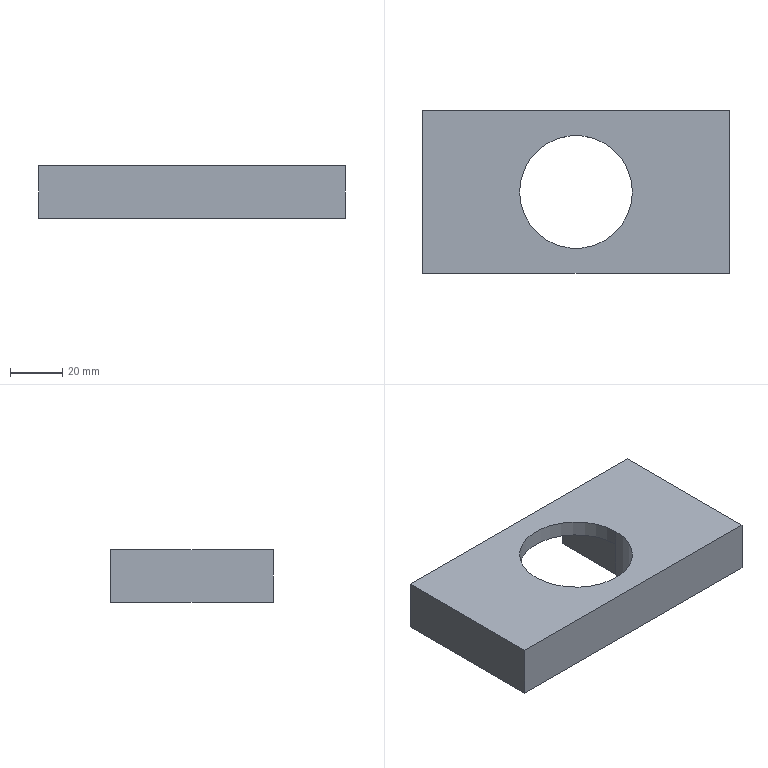Part | SolidWorks | features ICE 2, Chamfer 1, Extrusion 1 | 1 solid | 14 faces | box 117 x 62 x 20 mm | volume 107392 mm3 | plane 12 | cylinder 2 | commonest cylinder face diameters 43 x2
STEP:
#1=CARTESIAN_POINT('',(-21.5,0.,14.));
#2=VERTEX_POINT('',#1);
#3=CARTESIAN_POINT('',(-21.5,0.,0.));
#4=VERTEX_POINT('',#3);
#5=CARTESIAN_POINT('',(-21.5,0.,14.));
#6=DIRECTION('',(0.,0.,-1.));
#7=VECTOR('',#6,1000.);
#8=LINE('',#5,#7);
#9=EDGE_CURVE('',#2,#4,#8,.T.);
#10=ORIENTED_EDGE('',*,*,#9,.F.);
#11=CARTESIAN_POINT('',(-21.5,0.,20.));
#12=VERTEX_POINT('',#11);
#13=CARTESIAN_POINT('',(-21.5,0.,-0.001));
#14=DIRECTION('',(0.,0.,1.));
#15=VECTOR('',#14,1000.);
#16=LINE('',#13,#15);
#17=EDGE_CURVE('',#2,#12,#16,.T.);
#18=ORIENTED_EDGE('',*,*,#17,.T.);
#19=CARTESIAN_POINT('',(21.5,0.,20.));
#20=VERTEX_POINT('',#19);
#21=CARTESIAN_POINT('',(0.,0.,20.));
#22=DIRECTION('',(0.,0.,1.));
#23=DIRECTION('',(1.,0.,0.));
#24=AXIS2_PLACEMENT_3D('',#21,#22,#23);
#25=CIRCLE('',#24,21.5);
#26=EDGE_CURVE('',#12,#20,#25,.T.);
#27=ORIENTED_EDGE('',*,*,#26,.T.);
#28=CARTESIAN_POINT('',(21.5,0.,14.));
#29=VERTEX_POINT('',#28);
#30=CARTESIAN_POINT('',(21.5,0.,-0.001));
#31=DIRECTION('',(0.,0.,1.));
#32=VECTOR('',#31,1000.);
#33=LINE('',#30,#32);
#34=EDGE_CURVE('',#29,#20,#33,.T.);
#35=ORIENTED_EDGE('',*,*,#34,.F.);
#36=CARTESIAN_POINT('',(21.5,0.,0.));
#37=VERTEX_POINT('',#36);
#38=CARTESIAN_POINT('',(21.5,0.,14.));
#39=DIRECTION('',(0.,0.,-1.));
#40=VECTOR('',#39,1000.);
#41=LINE('',#38,#40);
#42=EDGE_CURVE('',#29,#37,#41,.T.);
#43=ORIENTED_EDGE('',*,*,#42,.T.);
#44=CARTESIAN_POINT('',(0.,0.,0.));
#45=DIRECTION('',(0.,0.,1.));
#46=DIRECTION('',(-1.,0.,0.));
#47=AXIS2_PLACEMENT_3D('',#44,#45,#46);
#48=CIRCLE('',#47,21.5);
#49=EDGE_CURVE('',#4,#37,#48,.T.);
#50=ORIENTED_EDGE('',*,*,#49,.F.);
#51=EDGE_LOOP('',(#10,#18,#27,#35,#43,#50));
#52=FACE_OUTER_BOUND('',#51,.T.);
#53=CARTESIAN_POINT('',(0.,0.,-0.001));
#54=DIRECTION('',(0.,0.,1.));
#55=DIRECTION('',(1.,0.,0.));
#56=AXIS2_PLACEMENT_3D('',#53,#54,#55);
#57=CYLINDRICAL_SURFACE('',#56,21.5);
#58=ADVANCED_FACE('',(#52),#57,.F.);
#59=CARTESIAN_POINT('',(58.5,-31.,0.));
#60=VERTEX_POINT('',#59);
#61=CARTESIAN_POINT('',(58.5,31.,0.));
#62=VERTEX_POINT('',#61);
#63=CARTESIAN_POINT('',(58.5,-31.,0.));
#64=DIRECTION('',(0.,1.,0.));
#65=VECTOR('',#64,1000.);
#66=LINE('',#63,#65);
#67=EDGE_CURVE('',#60,#62,#66,.T.);
#68=ORIENTED_EDGE('',*,*,#67,.T.);
#69=CARTESIAN_POINT('',(58.5,31.,20.));
#70=VERTEX_POINT('',#69);
#71=CARTESIAN_POINT('',(58.5,31.,20.));
#72=DIRECTION('',(0.,0.,-1.));
#73=VECTOR('',#72,1000.);
#74=LINE('',#71,#73);
#75=EDGE_CURVE('',#70,#62,#74,.T.);
#76=ORIENTED_EDGE('',*,*,#75,.F.);
#77=CARTESIAN_POINT('',(58.5,-31.,20.));
#78=VERTEX_POINT('',#77);
#79=CARTESIAN_POINT('',(58.5,-31.,20.));
#80=DIRECTION('',(0.,1.,0.));
#81=VECTOR('',#80,1000.);
#82=LINE('',#79,#81);
#83=EDGE_CURVE('',#78,#70,#82,.T.);
#84=ORIENTED_EDGE('',*,*,#83,.F.);
#85=CARTESIAN_POINT('',(58.5,-31.,20.));
#86=DIRECTION('',(0.,0.,-1.));
#87=VECTOR('',#86,1000.);
#88=LINE('',#85,#87);
#89=EDGE_CURVE('',#78,#60,#88,.T.);
#90=ORIENTED_EDGE('',*,*,#89,.T.);
#91=EDGE_LOOP('',(#68,#76,#84,#90));
#92=FACE_OUTER_BOUND('',#91,.T.);
#93=CARTESIAN_POINT('',(58.5,-31.,20.));
#94=DIRECTION('',(-1.,0.,0.));
#95=DIRECTION('',(0.,0.,1.));
#96=AXIS2_PLACEMENT_3D('',#93,#94,#95);
#97=PLANE('',#96);
#98=ADVANCED_FACE('',(#92),#97,.F.);
#99=CARTESIAN_POINT('',(23.5,31.,0.));
#100=VERTEX_POINT('',#99);
#101=CARTESIAN_POINT('',(-58.5,31.,0.));
#102=DIRECTION('',(-1.,0.,0.));
#103=VECTOR('',#102,1000.);
#104=LINE('',#101,#103);
#105=EDGE_CURVE('',#62,#100,#104,.T.);
#106=ORIENTED_EDGE('',*,*,#105,.T.);
#107=CARTESIAN_POINT('',(23.5,31.,16.));
#108=VERTEX_POINT('',#107);
#109=CARTESIAN_POINT('',(23.5,31.,20.));
#110=DIRECTION('',(0.,0.,1.));
#111=VECTOR('',#110,1000.);
#112=LINE('',#109,#111);
#113=EDGE_CURVE('',#100,#108,#112,.T.);
#114=ORIENTED_EDGE('',*,*,#113,.T.);
#115=CARTESIAN_POINT('',(-23.5,31.,16.));
#116=VERTEX_POINT('',#115);
#117=CARTESIAN_POINT('',(-21.5,31.,16.));
#118=DIRECTION('',(-1.,0.,0.));
#119=VECTOR('',#118,1000.);
#120=LINE('',#117,#119);
#121=EDGE_CURVE('',#108,#116,#120,.T.);
#122=ORIENTED_EDGE('',*,*,#121,.T.);
#123=CARTESIAN_POINT('',(-23.5,31.,0.));
#124=VERTEX_POINT('',#123);
#125=CARTESIAN_POINT('',(-23.5,31.,20.));
#126=DIRECTION('',(0.,0.,-1.));
#127=VECTOR('',#126,1000.);
#128=LINE('',#125,#127);
#129=EDGE_CURVE('',#116,#124,#128,.T.);
#130=ORIENTED_EDGE('',*,*,#129,.T.);
#131=CARTESIAN_POINT('',(-58.5,31.,0.));
#132=VERTEX_POINT('',#131);
#133=CARTESIAN_POINT('',(-58.5,31.,0.));
#134=DIRECTION('',(-1.,0.,0.));
#135=VECTOR('',#134,1000.);
#136=LINE('',#133,#135);
#137=EDGE_CURVE('',#124,#132,#136,.T.);
#138=ORIENTED_EDGE('',*,*,#137,.T.);
#139=CARTESIAN_POINT('',(-58.5,31.,20.));
#140=VERTEX_POINT('',#139);
#141=CARTESIAN_POINT('',(-58.5,31.,20.));
#142=DIRECTION('',(0.,0.,-1.));
#143=VECTOR('',#142,1000.);
#144=LINE('',#141,#143);
#145=EDGE_CURVE('',#140,#132,#144,.T.);
#146=ORIENTED_EDGE('',*,*,#145,.F.);
#147=CARTESIAN_POINT('',(-58.5,31.,20.));
#148=DIRECTION('',(-1.,0.,0.));
#149=VECTOR('',#148,1000.);
#150=LINE('',#147,#149);
#151=EDGE_CURVE('',#70,#140,#150,.T.);
#152=ORIENTED_EDGE('',*,*,#151,.F.);
#153=ORIENTED_EDGE('',*,*,#75,.T.);
#154=EDGE_LOOP('',(#106,#114,#122,#130,#138,#146,#152,#153));
#155=FACE_OUTER_BOUND('',#154,.T.);
#156=CARTESIAN_POINT('',(-58.5,31.,20.));
#157=DIRECTION('',(0.,-1.,0.));
#158=DIRECTION('',(0.,0.,-1.));
#159=AXIS2_PLACEMENT_3D('',#156,#157,#158);
#160=PLANE('',#159);
#161=ADVANCED_FACE('',(#155),#160,.F.);
#162=CARTESIAN_POINT('',(-58.5,-31.,0.));
#163=VERTEX_POINT('',#162);
#164=CARTESIAN_POINT('',(-58.5,-31.,0.));
#165=DIRECTION('',(0.,-1.,0.));
#166=VECTOR('',#165,1000.);
#167=LINE('',#164,#166);
#168=EDGE_CURVE('',#132,#163,#167,.T.);
#169=ORIENTED_EDGE('',*,*,#168,.T.);
#170=CARTESIAN_POINT('',(-58.5,-31.,20.));
#171=VERTEX_POINT('',#170);
#172=CARTESIAN_POINT('',(-58.5,-31.,20.));
#173=DIRECTION('',(0.,0.,-1.));
#174=VECTOR('',#173,1000.);
#175=LINE('',#172,#174);
#176=EDGE_CURVE('',#171,#163,#175,.T.);
#177=ORIENTED_EDGE('',*,*,#176,.F.);
#178=CARTESIAN_POINT('',(-58.5,-31.,20.));
#179=DIRECTION('',(0.,-1.,0.));
#180=VECTOR('',#179,1000.);
#181=LINE('',#178,#180);
#182=EDGE_CURVE('',#140,#171,#181,.T.);
#183=ORIENTED_EDGE('',*,*,#182,.F.);
#184=ORIENTED_EDGE('',*,*,#145,.T.);
#185=EDGE_LOOP('',(#169,#177,#183,#184));
#186=FACE_OUTER_BOUND('',#185,.T.);
#187=CARTESIAN_POINT('',(-58.5,-31.,20.));
#188=DIRECTION('',(1.,0.,0.));
#189=DIRECTION('',(0.,0.,-1.));
#190=AXIS2_PLACEMENT_3D('',#187,#188,#189);
#191=PLANE('',#190);
#192=ADVANCED_FACE('',(#186),#191,.F.);
#193=CARTESIAN_POINT('',(-58.5,-31.,0.));
#194=DIRECTION('',(1.,0.,0.));
#195=VECTOR('',#194,1000.);
#196=LINE('',#193,#195);
#197=EDGE_CURVE('',#163,#60,#196,.T.);
#198=ORIENTED_EDGE('',*,*,#197,.T.);
#199=ORIENTED_EDGE('',*,*,#89,.F.);
#200=CARTESIAN_POINT('',(-58.5,-31.,20.));
#201=DIRECTION('',(1.,0.,0.));
#202=VECTOR('',#201,1000.);
#203=LINE('',#200,#202);
#204=EDGE_CURVE('',#171,#78,#203,.T.);
#205=ORIENTED_EDGE('',*,*,#204,.F.);
#206=ORIENTED_EDGE('',*,*,#176,.T.);
#207=EDGE_LOOP('',(#198,#199,#205,#206));
#208=FACE_OUTER_BOUND('',#207,.T.);
#209=CARTESIAN_POINT('',(-58.5,-31.,20.));
#210=DIRECTION('',(0.,1.,0.));
#211=DIRECTION('',(0.,0.,1.));
#212=AXIS2_PLACEMENT_3D('',#209,#210,#211);
#213=PLANE('',#212);
#214=ADVANCED_FACE('',(#208),#213,.F.);
#215=CARTESIAN_POINT('',(0.,0.,20.));
#216=DIRECTION('',(0.,0.,1.));
#217=DIRECTION('',(1.,0.,0.));
#218=AXIS2_PLACEMENT_3D('',#215,#216,#217);
#219=CIRCLE('',#218,21.5);
#220=EDGE_CURVE('',#20,#12,#219,.T.);
#221=ORIENTED_EDGE('',*,*,#220,.F.);
#222=ORIENTED_EDGE('',*,*,#26,.F.);
#223=EDGE_LOOP('',(#221,#222));
#224=FACE_BOUND('',#223,.T.);
#225=ORIENTED_EDGE('',*,*,#83,.T.);
#226=ORIENTED_EDGE('',*,*,#151,.T.);
#227=ORIENTED_EDGE('',*,*,#182,.T.);
#228=ORIENTED_EDGE('',*,*,#204,.T.);
#229=EDGE_LOOP('',(#225,#226,#227,#228));
#230=FACE_OUTER_BOUND('',#229,.T.);
#231=CARTESIAN_POINT('',(0.,0.,20.));
#232=DIRECTION('',(0.,0.,-1.));
#233=DIRECTION('',(-1.,0.,0.));
#234=AXIS2_PLACEMENT_3D('',#231,#232,#233);
#235=PLANE('',#234);
#236=ADVANCED_FACE('',(#224,#230),#235,.F.);
#237=CARTESIAN_POINT('',(21.5,29.,0.));
#238=VERTEX_POINT('',#237);
#239=CARTESIAN_POINT('',(21.5,31.,0.));
#240=DIRECTION('',(0.,-1.,0.));
#241=VECTOR('',#240,1000.);
#242=LINE('',#239,#241);
#243=EDGE_CURVE('',#238,#37,#242,.T.);
#244=ORIENTED_EDGE('',*,*,#243,.F.);
#245=CARTESIAN_POINT('',(-3.75,3.75,0.));
#246=DIRECTION('',(0.7071,0.7071,0.));
#247=VECTOR('',#246,1000.);
#248=LINE('',#245,#247);
#249=EDGE_CURVE('',#238,#100,#248,.T.);
#250=ORIENTED_EDGE('',*,*,#249,.T.);
#251=ORIENTED_EDGE('',*,*,#105,.F.);
#252=ORIENTED_EDGE('',*,*,#67,.F.);
#253=ORIENTED_EDGE('',*,*,#197,.F.);
#254=ORIENTED_EDGE('',*,*,#168,.F.);
#255=ORIENTED_EDGE('',*,*,#137,.F.);
#256=CARTESIAN_POINT('',(-21.5,29.,0.));
#257=VERTEX_POINT('',#256);
#258=CARTESIAN_POINT('',(3.75,3.75,0.));
#259=DIRECTION('',(0.7071,-0.7071,0.));
#260=VECTOR('',#259,1000.);
#261=LINE('',#258,#260);
#262=EDGE_CURVE('',#124,#257,#261,.T.);
#263=ORIENTED_EDGE('',*,*,#262,.T.);
#264=CARTESIAN_POINT('',(-21.5,31.,0.));
#265=DIRECTION('',(0.,1.,0.));
#266=VECTOR('',#265,1000.);
#267=LINE('',#264,#266);
#268=EDGE_CURVE('',#4,#257,#267,.T.);
#269=ORIENTED_EDGE('',*,*,#268,.F.);
#270=ORIENTED_EDGE('',*,*,#49,.T.);
#271=EDGE_LOOP('',(#244,#250,#251,#252,#253,#254,#255,#263,#269,#270));
#272=FACE_OUTER_BOUND('',#271,.T.);
#273=CARTESIAN_POINT('',(0.,0.,0.));
#274=DIRECTION('',(0.,0.,-1.));
#275=DIRECTION('',(-1.,0.,0.));
#276=AXIS2_PLACEMENT_3D('',#273,#274,#275);
#277=PLANE('',#276);
#278=ADVANCED_FACE('',(#272),#277,.T.);
#279=ORIENTED_EDGE('',*,*,#17,.F.);
#280=CARTESIAN_POINT('',(0.,0.,14.));
#281=DIRECTION('',(0.,0.,1.));
#282=DIRECTION('',(-1.,0.,0.));
#283=AXIS2_PLACEMENT_3D('',#280,#281,#282);
#284=CIRCLE('',#283,21.5);
#285=EDGE_CURVE('',#29,#2,#284,.T.);
#286=ORIENTED_EDGE('',*,*,#285,.F.);
#287=ORIENTED_EDGE('',*,*,#34,.T.);
#288=ORIENTED_EDGE('',*,*,#220,.T.);
#289=EDGE_LOOP('',(#279,#286,#287,#288));
#290=FACE_OUTER_BOUND('',#289,.T.);
#291=CARTESIAN_POINT('',(0.,0.,-0.001));
#292=DIRECTION('',(0.,0.,1.));
#293=DIRECTION('',(1.,0.,0.));
#294=AXIS2_PLACEMENT_3D('',#291,#292,#293);
#295=CYLINDRICAL_SURFACE('',#294,21.5);
#296=ADVANCED_FACE('',(#290),#295,.F.);
#297=CARTESIAN_POINT('',(-21.5,29.,14.));
#298=VERTEX_POINT('',#297);
#299=CARTESIAN_POINT('',(-21.5,31.,14.));
#300=DIRECTION('',(0.,1.,0.));
#301=VECTOR('',#300,1000.);
#302=LINE('',#299,#301);
#303=EDGE_CURVE('',#2,#298,#302,.T.);
#304=ORIENTED_EDGE('',*,*,#303,.T.);
#305=CARTESIAN_POINT('',(21.5,29.,14.));
#306=VERTEX_POINT('',#305);
#307=CARTESIAN_POINT('',(21.5,29.,14.));
#308=DIRECTION('',(1.,0.,0.));
#309=VECTOR('',#308,1000.);
#310=LINE('',#307,#309);
#311=EDGE_CURVE('',#298,#306,#310,.T.);
#312=ORIENTED_EDGE('',*,*,#311,.T.);
#313=CARTESIAN_POINT('',(21.5,31.,14.));
#314=DIRECTION('',(0.,-1.,0.));
#315=VECTOR('',#314,1000.);
#316=LINE('',#313,#315);
#317=EDGE_CURVE('',#306,#29,#316,.T.);
#318=ORIENTED_EDGE('',*,*,#317,.T.);
#319=ORIENTED_EDGE('',*,*,#285,.T.);
#320=EDGE_LOOP('',(#304,#312,#318,#319));
#321=FACE_OUTER_BOUND('',#320,.T.);
#322=CARTESIAN_POINT('',(0.,0.,14.));
#323=DIRECTION('',(0.,0.,-1.));
#324=DIRECTION('',(-1.,0.,0.));
#325=AXIS2_PLACEMENT_3D('',#322,#323,#324);
#326=PLANE('',#325);
#327=ADVANCED_FACE('',(#321),#326,.T.);
#328=ORIENTED_EDGE('',*,*,#317,.F.);
#329=CARTESIAN_POINT('',(21.5,29.,14.));
#330=DIRECTION('',(0.,0.,-1.));
#331=VECTOR('',#330,1000.);
#332=LINE('',#329,#331);
#333=EDGE_CURVE('',#306,#238,#332,.T.);
#334=ORIENTED_EDGE('',*,*,#333,.T.);
#335=ORIENTED_EDGE('',*,*,#243,.T.);
#336=ORIENTED_EDGE('',*,*,#42,.F.);
#337=EDGE_LOOP('',(#328,#334,#335,#336));
#338=FACE_OUTER_BOUND('',#337,.T.);
#339=CARTESIAN_POINT('',(21.5,31.,14.));
#340=DIRECTION('',(1.,0.,0.));
#341=DIRECTION('',(0.,0.,-1.));
#342=AXIS2_PLACEMENT_3D('',#339,#340,#341);
#343=PLANE('',#342);
#344=ADVANCED_FACE('',(#338),#343,.F.);
#345=ORIENTED_EDGE('',*,*,#268,.T.);
#346=CARTESIAN_POINT('',(-21.5,29.,14.));
#347=DIRECTION('',(0.,0.,1.));
#348=VECTOR('',#347,1000.);
#349=LINE('',#346,#348);
#350=EDGE_CURVE('',#257,#298,#349,.T.);
#351=ORIENTED_EDGE('',*,*,#350,.T.);
#352=ORIENTED_EDGE('',*,*,#303,.F.);
#353=ORIENTED_EDGE('',*,*,#9,.T.);
#354=EDGE_LOOP('',(#345,#351,#352,#353));
#355=FACE_OUTER_BOUND('',#354,.T.);
#356=CARTESIAN_POINT('',(-21.5,31.,14.));
#357=DIRECTION('',(-1.,0.,0.));
#358=DIRECTION('',(0.,0.,1.));
#359=AXIS2_PLACEMENT_3D('',#356,#357,#358);
#360=PLANE('',#359);
#361=ADVANCED_FACE('',(#355),#360,.F.);
#362=ORIENTED_EDGE('',*,*,#262,.F.);
#363=ORIENTED_EDGE('',*,*,#129,.F.);
#364=CARTESIAN_POINT('',(-24.833,32.333,17.333));
#365=DIRECTION('',(-0.5774,0.5774,0.5774));
#366=VECTOR('',#365,1000.);
#367=LINE('',#364,#366);
#368=EDGE_CURVE('',#298,#116,#367,.T.);
#369=ORIENTED_EDGE('',*,*,#368,.F.);
#370=ORIENTED_EDGE('',*,*,#350,.F.);
#371=EDGE_LOOP('',(#362,#363,#369,#370));
#372=FACE_OUTER_BOUND('',#371,.T.);
#373=CARTESIAN_POINT('',(-23.5,31.,20.));
#374=DIRECTION('',(-0.7071,-0.7071,0.));
#375=DIRECTION('',(0.,0.,-1.));
#376=AXIS2_PLACEMENT_3D('',#373,#374,#375);
#377=PLANE('',#376);
#378=ADVANCED_FACE('',(#372),#377,.F.);
#379=ORIENTED_EDGE('',*,*,#368,.T.);
#380=ORIENTED_EDGE('',*,*,#121,.F.);
#381=CARTESIAN_POINT('',(21.5,29.,14.));
#382=DIRECTION('',(0.5774,0.5774,0.5774));
#383=VECTOR('',#382,1000.);
#384=LINE('',#381,#383);
#385=EDGE_CURVE('',#306,#108,#384,.T.);
#386=ORIENTED_EDGE('',*,*,#385,.F.);
#387=ORIENTED_EDGE('',*,*,#311,.F.);
#388=EDGE_LOOP('',(#379,#380,#386,#387));
#389=FACE_OUTER_BOUND('',#388,.T.);
#390=CARTESIAN_POINT('',(0.,29.,14.));
#391=DIRECTION('',(0.,0.7071,-0.7071));
#392=DIRECTION('',(-1.,0.,0.));
#393=AXIS2_PLACEMENT_3D('',#390,#391,#392);
#394=PLANE('',#393);
#395=ADVANCED_FACE('',(#389),#394,.T.);
#396=ORIENTED_EDGE('',*,*,#385,.T.);
#397=ORIENTED_EDGE('',*,*,#113,.F.);
#398=ORIENTED_EDGE('',*,*,#249,.F.);
#399=ORIENTED_EDGE('',*,*,#333,.F.);
#400=EDGE_LOOP('',(#396,#397,#398,#399));
#401=FACE_OUTER_BOUND('',#400,.T.);
#402=CARTESIAN_POINT('',(21.5,29.,14.));
#403=DIRECTION('',(0.7071,-0.7071,0.));
#404=DIRECTION('',(0.,0.,-1.));
#405=AXIS2_PLACEMENT_3D('',#402,#403,#404);
#406=PLANE('',#405);
#407=ADVANCED_FACE('',(#401),#406,.F.);
#408=CLOSED_SHELL('',(#58,#98,#161,#192,#214,#236,#278,#296,#327,#344,#361,#378,#395,#407));
#409=MANIFOLD_SOLID_BREP('',#408);
#410=CARTESIAN_POINT('',(0.,0.,0.));
#411=DIRECTION('',(0.,0.,1.));
#412=DIRECTION('',(1.,0.,0.));
#413=AXIS2_PLACEMENT_3D('',#410,#411,#412);
#414=(LENGTH_UNIT()NAMED_UNIT(*)SI_UNIT(.MILLI.,.METRE.));
#415=UNCERTAINTY_MEASURE_WITH_UNIT(LENGTH_MEASURE(0.00001),#414,'','');
#416=(NAMED_UNIT(*)PLANE_ANGLE_UNIT()SI_UNIT($,.RADIAN.));
#417=(NAMED_UNIT(*)SI_UNIT($,.STERADIAN.)SOLID_ANGLE_UNIT());
#418=(GEOMETRIC_REPRESENTATION_CONTEXT(3)GLOBAL_UNCERTAINTY_ASSIGNED_CONTEXT((#415))GLOBAL_UNIT_ASSIGNED_CONTEXT((#414,#416,#417))REPRESENTATION_CONTEXT('',''));
#419=ADVANCED_BREP_SHAPE_REPRESENTATION('',(#409,#413),#418);